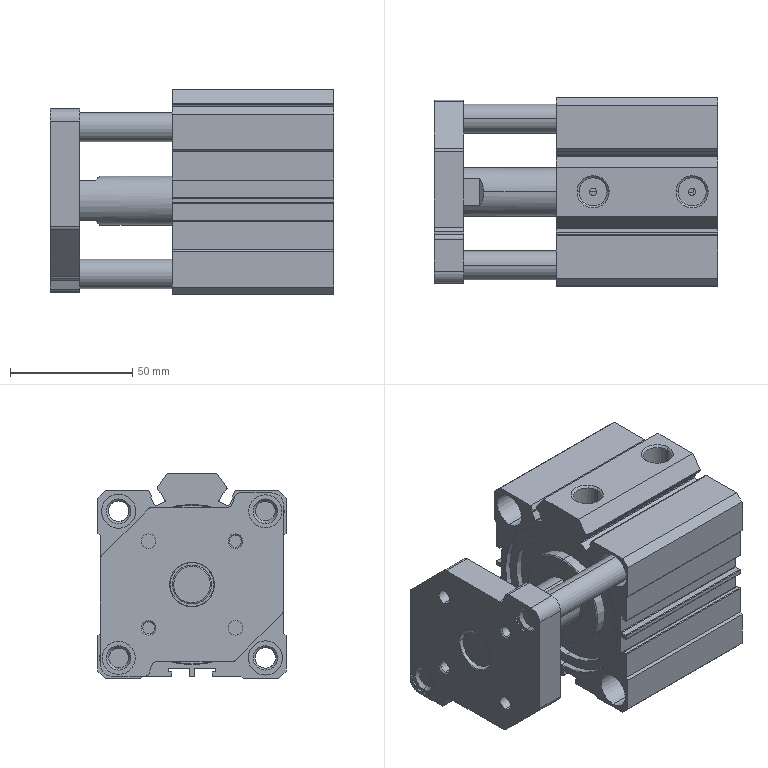Part | SolidWorks | 2 solids | 324 faces | box 116 x 77 x 84 mm | volume 320960 mm3 | cylinder 147 | plane 125 | cone 44 | spline 8 | commonest cylinder face diameters 0.4 x41 0.8 x8 4 x8 8.376 x8 12 x8 14 x8